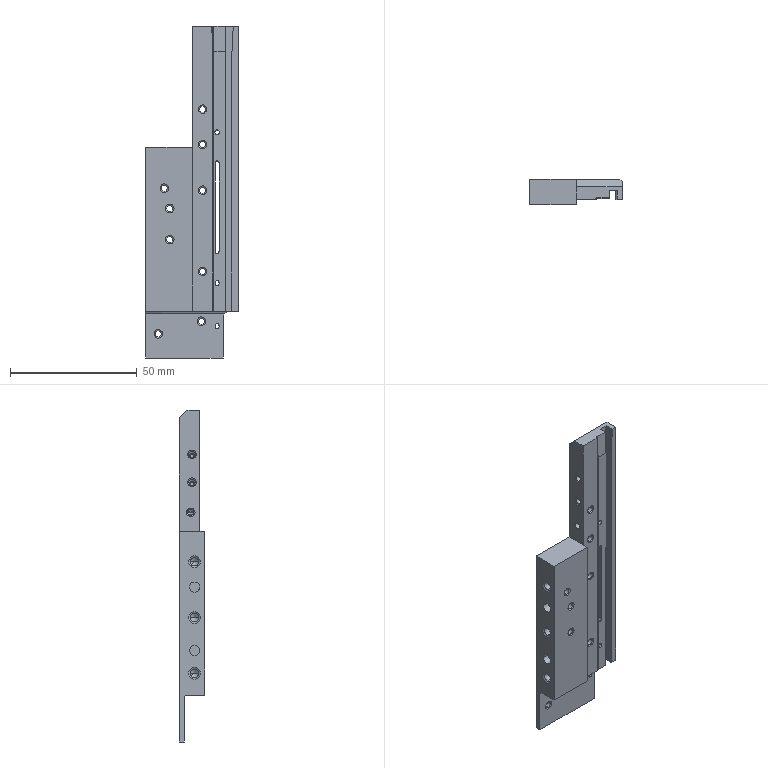Part | NX | 1 solid | 124 faces | box 36.55 x 10 x 131 mm | volume 26389 mm3 | cylinder 47 | cone 42 | plane 35 | commonest cylinder face diameters 2.5 x24 1.5 x9 3.3 x6 4 x4 1.8 x2 2 x1